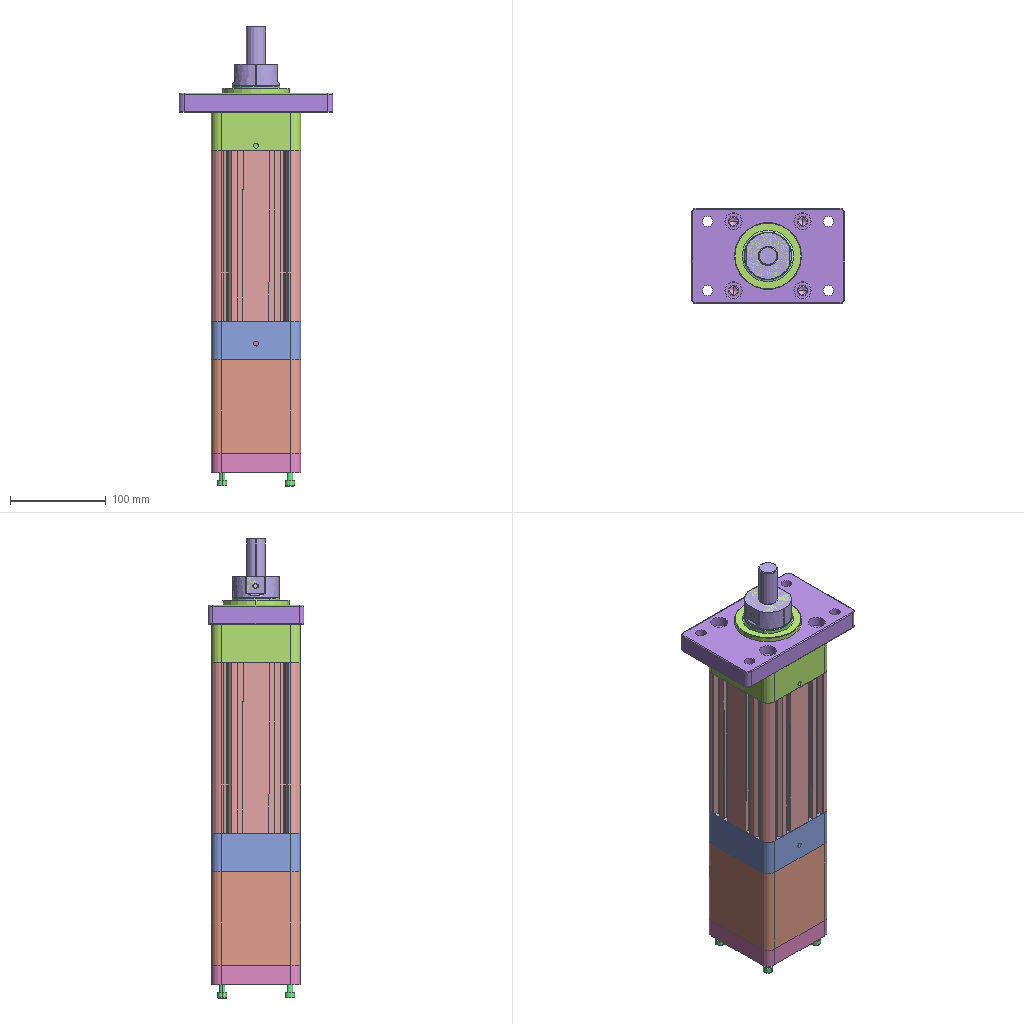Assembly | SolidWorks | 20 different items | 34 placed | box 160 x 100 x 480 mm
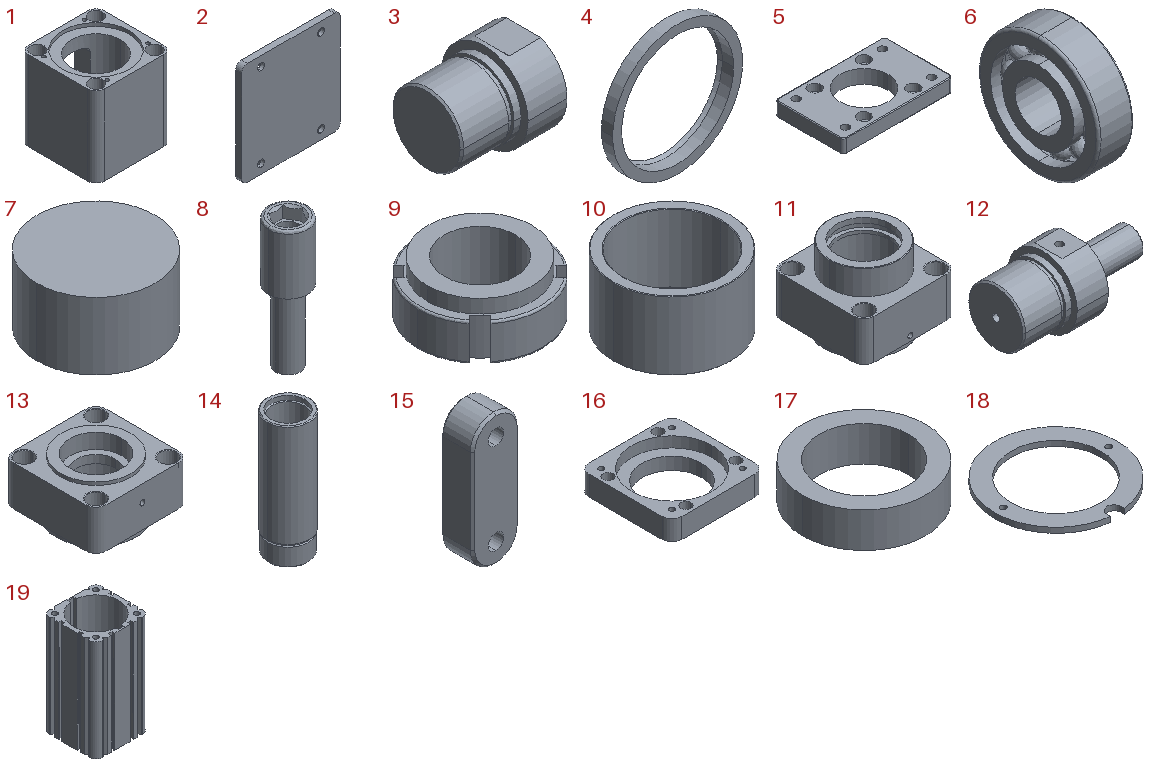Parts list (item | name | quantity | size | volume | features):
1 | - | x1 | 93 x 93 x 98 mm | 432719 mm3 | features ICE 5, HoleWzd 4, Fillet 3, CirPattern 1, Extrusion 1
2 | - | x1 | 49.5 x 3 x 51.5 mm | 7470 mm3 | features Chamfer 1, Extrusion 1, Fillet 1
3 | - | x1 | 55 x 49 x 49 mm | 69401 mm3 | features ICE 5, BaseBody 1, Chamfer 1, HoleWzd 1, MoveFace 1
4 | - | x1 | 58 x 6.5 x 58 mm | 3817 mm3 | features Revolution 1
5 | - | x1 | 160 x 100 x 20 mm | 213466 mm3 | features Fillet 2, HoleWzd 2, Extrusion 1
6 | - | x3 | 15 x 52 x 52 mm | 18286 mm3 | features Revolution 3, Fillet 2, CirPattern 1
7 | - | x3 | 8.8 x 8.8 x 5 mm | 304.106 mm3 | features Extrusion 1
8 | - | x8 | 16 x 16 x 53 mm | 5579 mm3 | features ICE 2, BaseBody 1
9 | - | x1 | 32 x 32 x 13 mm | 5836 mm3 | features BaseBody 1, MoveFace 1
10 | - | x1 | 60 x 60 x 35 mm | 30207 mm3 | features Chamfer 1, Extrusion 1
11 | - | x1 | 93 x 93 x 75 mm | 240309 mm3 | features ICE 6, BaseBody 1, HoleWzd 1
12 | - | x2 | 95 x 49 x 49 mm | 93064 mm3 | features ICE 4, Chamfer 2, BaseBody 1, MoveFace 1
13 | - | x1 | 93 x 93 x 53 mm | 265876 mm3 | features ICE 4, HoleWzd 3, BaseBody 1, MoveFace 1
14 | - | x1 | 50 x 50 x 147 mm | 134333 mm3 | features Chamfer 4, RevCut 2, Extrusion 1, ICE 1
15 | - | x2 | 10.3 x 7 x 29 mm | 1657 mm3 | features Fillet 2, ICE 2, Chamfer 1, Extrusion 1, HoleWzd 1
16 | - | x1 | 93 x 93 x 23 mm | 93388 mm3 | features HoleWzd 3, CirPattern 2, ICE 2, Extrusion 1, Fillet 1
17 | - | x2 | 28 x 28 x 8 mm | 2362 mm3 | features Extrusion 1
18 | - | x1 | 70 x 69.771 x 3 mm | 5244 mm3 | features ICE 4, Extrusion 1, HoleWzd 1
19 | - | x1 | 93 x 93 x 178 mm | 509573 mm3 | features ICE 6, CirPattern 4, Fillet 3, Extrusion 1, HoleWzd 1
20 | hexagon socket head cap screws gb | x1 | - | - | -
Mates (type | each side: item.copy, entity, surface, feature):
Concentric | 19.1 face cylinder Boss-Extrude1 | 11.1 face cylinder Import 1
Coincident | 19.1 face plane Boss-Extrude1 | 11.1 face plane Import 1
Concentric | 19.1 face cylinder Cut-Extrude3 | 8.1 face cylinder Import 1
Concentric | 13.1 face cylinder Import 1 | 6.1 face cylinder Boss-Revolve2
Coincident | 13.1 face plane Import 1 | 6.1 face plane Base-Revolve
Coincident | 13.1 face plane Import 1 | 6.2 face plane Boss-Revolve2
Concentric | 13.1 face cylinder Import 1 | 6.2 face cylinder Base-Revolve
Concentric | 13.1 face cylinder Import 1 | 6.3 face cylinder Base-Revolve
Coincident | 6.2 face plane Base-Revolve | 6.3 face plane Base-Revolve
Concentric | 19.1 face cylinder Boss-Extrude1 | 13.1 face cylinder Import 1
Concentric | 19.1 face cylinder Cut-Extrude3 | 13.1 face cylinder Import 1
Coincident | 19.1 face plane Boss-Extrude1 | 13.1 face plane Import 1
Concentric | 13.1 face cylinder Import 1 | 8.2 face cylinder Import 1
Coincident | 11.1 face plane Import 1 | 8.1 face plane Cut-Extrude2
Coincident | 13.1 face plane Import 1 | 8.2 face plane Cut-Extrude2
Coincident | 6.1 face plane Boss-Revolve2 | 17.1 face plane Boss-Extrude1
Coincident | 6.1 face plane Boss-Revolve2 | 17.2 face plane Boss-Extrude1
Coincident | 9.1 face plane Import 1 | 17.2 face plane Boss-Extrude1
Concentric | 11.1 face cylinder Import 1 | 7.1 face cylinder Boss-Extrude1
Concentric | 19.1 face cylinder Cut-Extrude3 | 11.1 face cylinder Import 1
Concentric | 13.1 face cylinder Import 1 | 7.2 face cylinder Boss-Extrude1
Concentric | 11.1 face cylinder Cut-Extrude1 | 10.1 face cylinder Boss-Extrude1
Coincident | 11.1 face plane Import 1 | 10.1 face plane Boss-Extrude1
Concentric | 14.1 face cylinder Boss-Extrude1 | 4.1 face cylinder Revolve1
Coincident | 11.1 face plane Import 1 | 4.1 face plane Revolve1
Concentric | 12.1 face cylinder Import 1 | 14.1 face cylinder Cut-Revolve2
Coincident | 12.1 face plane Import 1 | 14.1 face plane Boss-Extrude1
Concentric | 11.1 face cylinder Import 1 | assembly face
Concentric | 13.1 face cylinder Import 1 | 1.1 face cylinder Cut-Extrude1
Coincident | 13.1 face plane Import 1 | 1.1 face plane Boss-Extrude1
Width | 1.1 face plane Cut-Extrude5 | 1.1 face plane Cut-Extrude5 | 2.1 face plane Boss-Extrude1 | 2.1 face plane Boss-Extrude1
Width | 1.1 face plane Cut-Extrude3 | 1.1 face plane Cut-Extrude3 | 2.1 face plane Boss-Extrude1 | 2.1 face plane Boss-Extrude1
Coincident | 1.1 face plane Cut-Extrude5 | 2.1 face plane Boss-Extrude1
DistanceDim | 12.1 face plane Import 1 | 11.1 face plane Import 1
Concentric | 12.1 face cylinder Import 1 | 3.1 face cylinder Import 1
Coincident | 12.1 face plane Import 1 | 3.1 face plane Import 1 | 2 times
Concentric | 1.1 face cylinder Cut-Extrude2 | 16.1 face cylinder Boss-Extrude1
Parallel | 1.1 face plane Boss-Extrude1 | 16.1 face plane Boss-Extrude1
Coincident | 1.1 face plane Boss-Extrude1 | 16.1 face plane Boss-Extrude1
Concentric | assembly face | 16.1 face cylinder Cut-Extrude1
Coincident | assembly face | 16.1 face plane Boss-Extrude1
Concentric | 13.1 face cylinder Import 1 | 18.1 face cylinder Boss-Extrude1
Concentric | 13.1 face cylinder M3 Tapped Hole2 | 18.1 face cylinder Cut-Extrude4
Coincident | 13.1 face plane Import 1 | 18.1 face plane Boss-Extrude1
Coincident | 13.1 face plane Cut-Extrude2 | 7.2 face plane Boss-Extrude1
Concentric | 13.1 face cylinder Import 1 | 1.1 face cylinder CBORE for M10 Hex Head Bolt1
Coincident | 11.1 face plane Cut-Extrude5 | 7.1 face plane Boss-Extrude1
Concentric | 1.1 face cylinder Cut-Extrude4 | assembly face
Concentric | 1.1 face cylinder M5 Tapped Hole2 | assembly face
Coincident | 1.1 face plane Boss-Extrude1 | assembly face
Concentric | assembly face | assembly face | 3 times
Coincident | assembly face | assembly face | 2 times
Parallel | assembly face | assembly face
Concentric | assembly face | 16.1 face cylinder M6 Tapped Hole1
Concentric | 14.1 edge | 12.2 face cylinder Import 1
Coincident | 14.1 face plane Boss-Extrude1 | 12.2 face plane Import 1
Coincident | 19.1 face plane Cut-Extrude4 | assembly edge
Concentric | 19.1 face cylinder M10x1.0 Tapped Hole1 | 7.3 face cylinder Boss-Extrude1
Coincident | 19.1 face plane Boss-Extrude1 | 7.3 face plane Boss-Extrude1
Concentric | 11.1 face cylinder Import 1 | 5.1 face cylinder Boss-Extrude1
Parallel | 11.1 face plane Cut-Extrude5 | 5.1 face plane Boss-Extrude1
Coincident | 11.1 face plane Import 1 | 5.1 face plane Boss-Extrude1